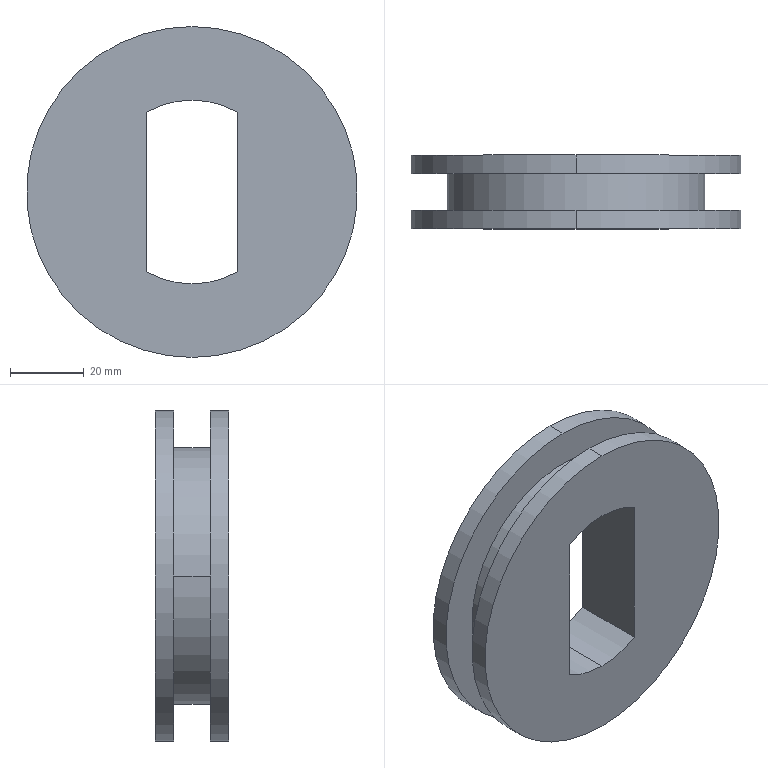Part | SolidWorks | 1 solid | 15 faces | box 90 x 20 x 90 mm | volume 78186 mm3 | cylinder 9 | plane 6 | commonest cylinder face diameters 90 x4 50 x3 70 x2
STEP:
#1=CARTESIAN_POINT('',(-35.,-5.,0.));
#2=VERTEX_POINT('',#1);
#3=CARTESIAN_POINT('',(35.,-5.,0.));
#4=VERTEX_POINT('',#3);
#5=CARTESIAN_POINT('',(0.,-5.,0.));
#6=DIRECTION('',(0.,1.,0.));
#7=DIRECTION('',(-1.,0.,0.));
#8=AXIS2_PLACEMENT_3D('',#5,#6,#7);
#9=CIRCLE('',#8,35.);
#10=EDGE_CURVE('',#2,#4,#9,.T.);
#11=ORIENTED_EDGE('',*,*,#10,.T.);
#12=CARTESIAN_POINT('',(35.,5.,0.));
#13=VERTEX_POINT('',#12);
#14=CARTESIAN_POINT('',(35.,10.,0.));
#15=DIRECTION('',(0.,1.,0.));
#16=VECTOR('',#15,1000.);
#17=LINE('',#14,#16);
#18=EDGE_CURVE('',#4,#13,#17,.T.);
#19=ORIENTED_EDGE('',*,*,#18,.T.);
#20=CARTESIAN_POINT('',(-35.,5.,0.));
#21=VERTEX_POINT('',#20);
#22=CARTESIAN_POINT('',(0.,5.,0.));
#23=DIRECTION('',(0.,1.,0.));
#24=DIRECTION('',(-1.,0.,0.));
#25=AXIS2_PLACEMENT_3D('',#22,#23,#24);
#26=CIRCLE('',#25,35.);
#27=EDGE_CURVE('',#21,#13,#26,.T.);
#28=ORIENTED_EDGE('',*,*,#27,.F.);
#29=CARTESIAN_POINT('',(-35.,10.,0.));
#30=DIRECTION('',(0.,1.,0.));
#31=VECTOR('',#30,1000.);
#32=LINE('',#29,#31);
#33=EDGE_CURVE('',#2,#21,#32,.T.);
#34=ORIENTED_EDGE('',*,*,#33,.F.);
#35=EDGE_LOOP('',(#11,#19,#28,#34));
#36=FACE_OUTER_BOUND('',#35,.T.);
#37=CARTESIAN_POINT('',(0.,10.,0.));
#38=DIRECTION('',(0.,1.,0.));
#39=DIRECTION('',(-1.,0.,0.));
#40=AXIS2_PLACEMENT_3D('',#37,#38,#39);
#41=CYLINDRICAL_SURFACE('',#40,35.);
#42=ADVANCED_FACE('',(#36),#41,.T.);
#43=CARTESIAN_POINT('',(12.5,10.,-21.651));
#44=VERTEX_POINT('',#43);
#45=CARTESIAN_POINT('',(0.,10.,-25.));
#46=VERTEX_POINT('',#45);
#47=CARTESIAN_POINT('',(0.,10.,0.));
#48=DIRECTION('',(0.,1.,0.));
#49=DIRECTION('',(0.,0.,1.));
#50=AXIS2_PLACEMENT_3D('',#47,#48,#49);
#51=CIRCLE('',#50,25.);
#52=EDGE_CURVE('',#44,#46,#51,.T.);
#53=ORIENTED_EDGE('',*,*,#52,.T.);
#54=CARTESIAN_POINT('',(0.,-10.,-25.));
#55=VERTEX_POINT('',#54);
#56=CARTESIAN_POINT('',(0.,10.,-25.));
#57=DIRECTION('',(0.,-1.,0.));
#58=VECTOR('',#57,1000.);
#59=LINE('',#56,#58);
#60=EDGE_CURVE('',#46,#55,#59,.T.);
#61=ORIENTED_EDGE('',*,*,#60,.T.);
#62=CARTESIAN_POINT('',(12.5,-10.,-21.651));
#63=VERTEX_POINT('',#62);
#64=CARTESIAN_POINT('',(0.,-10.,0.));
#65=DIRECTION('',(0.,1.,0.));
#66=DIRECTION('',(0.,0.,1.));
#67=AXIS2_PLACEMENT_3D('',#64,#65,#66);
#68=CIRCLE('',#67,25.);
#69=EDGE_CURVE('',#63,#55,#68,.T.);
#70=ORIENTED_EDGE('',*,*,#69,.F.);
#71=CARTESIAN_POINT('',(12.5,10.,-21.651));
#72=DIRECTION('',(0.,-1.,0.));
#73=VECTOR('',#72,1000.);
#74=LINE('',#71,#73);
#75=EDGE_CURVE('',#44,#63,#74,.T.);
#76=ORIENTED_EDGE('',*,*,#75,.F.);
#77=EDGE_LOOP('',(#53,#61,#70,#76));
#78=FACE_OUTER_BOUND('',#77,.T.);
#79=CARTESIAN_POINT('',(0.,10.,0.));
#80=DIRECTION('',(0.,-1.,0.));
#81=DIRECTION('',(0.,0.,-1.));
#82=AXIS2_PLACEMENT_3D('',#79,#80,#81);
#83=CYLINDRICAL_SURFACE('',#82,25.);
#84=ADVANCED_FACE('',(#78),#83,.F.);
#85=CARTESIAN_POINT('',(0.,-5.,45.));
#86=VERTEX_POINT('',#85);
#87=CARTESIAN_POINT('',(0.,-5.,-45.));
#88=VERTEX_POINT('',#87);
#89=CARTESIAN_POINT('',(0.,-5.,0.));
#90=DIRECTION('',(0.,1.,0.));
#91=DIRECTION('',(-1.,0.,0.));
#92=AXIS2_PLACEMENT_3D('',#89,#90,#91);
#93=CIRCLE('',#92,45.);
#94=EDGE_CURVE('',#86,#88,#93,.T.);
#95=ORIENTED_EDGE('',*,*,#94,.F.);
#96=CARTESIAN_POINT('',(0.,-10.,45.));
#97=VERTEX_POINT('',#96);
#98=CARTESIAN_POINT('',(0.,10.,45.));
#99=DIRECTION('',(0.,-1.,0.));
#100=VECTOR('',#99,1000.);
#101=LINE('',#98,#100);
#102=EDGE_CURVE('',#86,#97,#101,.T.);
#103=ORIENTED_EDGE('',*,*,#102,.T.);
#104=CARTESIAN_POINT('',(0.,-10.,-45.));
#105=VERTEX_POINT('',#104);
#106=CARTESIAN_POINT('',(0.,-10.,0.));
#107=DIRECTION('',(0.,1.,0.));
#108=DIRECTION('',(0.,0.,1.));
#109=AXIS2_PLACEMENT_3D('',#106,#107,#108);
#110=CIRCLE('',#109,45.);
#111=EDGE_CURVE('',#97,#105,#110,.T.);
#112=ORIENTED_EDGE('',*,*,#111,.T.);
#113=CARTESIAN_POINT('',(0.,10.,-45.));
#114=DIRECTION('',(0.,-1.,0.));
#115=VECTOR('',#114,1000.);
#116=LINE('',#113,#115);
#117=EDGE_CURVE('',#88,#105,#116,.T.);
#118=ORIENTED_EDGE('',*,*,#117,.F.);
#119=EDGE_LOOP('',(#95,#103,#112,#118));
#120=FACE_OUTER_BOUND('',#119,.T.);
#121=CARTESIAN_POINT('',(0.,10.,0.));
#122=DIRECTION('',(0.,-1.,0.));
#123=DIRECTION('',(0.,0.,-1.));
#124=AXIS2_PLACEMENT_3D('',#121,#122,#123);
#125=CYLINDRICAL_SURFACE('',#124,45.);
#126=ADVANCED_FACE('',(#120),#125,.T.);
#127=CARTESIAN_POINT('',(0.,10.,45.));
#128=VERTEX_POINT('',#127);
#129=CARTESIAN_POINT('',(0.,10.,-45.));
#130=VERTEX_POINT('',#129);
#131=CARTESIAN_POINT('',(0.,10.,0.));
#132=DIRECTION('',(0.,1.,0.));
#133=DIRECTION('',(0.,0.,1.));
#134=AXIS2_PLACEMENT_3D('',#131,#132,#133);
#135=CIRCLE('',#134,45.);
#136=EDGE_CURVE('',#128,#130,#135,.T.);
#137=ORIENTED_EDGE('',*,*,#136,.F.);
#138=CARTESIAN_POINT('',(0.,5.,45.));
#139=VERTEX_POINT('',#138);
#140=CARTESIAN_POINT('',(0.,10.,45.));
#141=DIRECTION('',(0.,-1.,0.));
#142=VECTOR('',#141,1000.);
#143=LINE('',#140,#142);
#144=EDGE_CURVE('',#128,#139,#143,.T.);
#145=ORIENTED_EDGE('',*,*,#144,.T.);
#146=CARTESIAN_POINT('',(0.,5.,-45.));
#147=VERTEX_POINT('',#146);
#148=CARTESIAN_POINT('',(0.,5.,0.));
#149=DIRECTION('',(0.,-1.,0.));
#150=DIRECTION('',(1.,0.,0.));
#151=AXIS2_PLACEMENT_3D('',#148,#149,#150);
#152=CIRCLE('',#151,45.);
#153=EDGE_CURVE('',#147,#139,#152,.T.);
#154=ORIENTED_EDGE('',*,*,#153,.F.);
#155=CARTESIAN_POINT('',(0.,10.,-45.));
#156=DIRECTION('',(0.,-1.,0.));
#157=VECTOR('',#156,1000.);
#158=LINE('',#155,#157);
#159=EDGE_CURVE('',#130,#147,#158,.T.);
#160=ORIENTED_EDGE('',*,*,#159,.F.);
#161=EDGE_LOOP('',(#137,#145,#154,#160));
#162=FACE_OUTER_BOUND('',#161,.T.);
#163=CARTESIAN_POINT('',(0.,10.,0.));
#164=DIRECTION('',(0.,-1.,0.));
#165=DIRECTION('',(0.,0.,-1.));
#166=AXIS2_PLACEMENT_3D('',#163,#164,#165);
#167=CYLINDRICAL_SURFACE('',#166,45.);
#168=ADVANCED_FACE('',(#162),#167,.T.);
#169=ORIENTED_EDGE('',*,*,#144,.F.);
#170=CARTESIAN_POINT('',(0.,10.,0.));
#171=DIRECTION('',(0.,1.,0.));
#172=DIRECTION('',(0.,0.,1.));
#173=AXIS2_PLACEMENT_3D('',#170,#171,#172);
#174=CIRCLE('',#173,45.);
#175=EDGE_CURVE('',#130,#128,#174,.T.);
#176=ORIENTED_EDGE('',*,*,#175,.F.);
#177=ORIENTED_EDGE('',*,*,#159,.T.);
#178=CARTESIAN_POINT('',(0.,5.,0.));
#179=DIRECTION('',(0.,-1.,0.));
#180=DIRECTION('',(1.,0.,0.));
#181=AXIS2_PLACEMENT_3D('',#178,#179,#180);
#182=CIRCLE('',#181,45.);
#183=EDGE_CURVE('',#139,#147,#182,.T.);
#184=ORIENTED_EDGE('',*,*,#183,.F.);
#185=EDGE_LOOP('',(#169,#176,#177,#184));
#186=FACE_OUTER_BOUND('',#185,.T.);
#187=CARTESIAN_POINT('',(0.,10.,0.));
#188=DIRECTION('',(0.,-1.,0.));
#189=DIRECTION('',(0.,0.,-1.));
#190=AXIS2_PLACEMENT_3D('',#187,#188,#189);
#191=CYLINDRICAL_SURFACE('',#190,45.);
#192=ADVANCED_FACE('',(#186),#191,.T.);
#193=ORIENTED_EDGE('',*,*,#102,.F.);
#194=CARTESIAN_POINT('',(0.,-5.,0.));
#195=DIRECTION('',(0.,1.,0.));
#196=DIRECTION('',(-1.,0.,0.));
#197=AXIS2_PLACEMENT_3D('',#194,#195,#196);
#198=CIRCLE('',#197,45.);
#199=EDGE_CURVE('',#88,#86,#198,.T.);
#200=ORIENTED_EDGE('',*,*,#199,.F.);
#201=ORIENTED_EDGE('',*,*,#117,.T.);
#202=CARTESIAN_POINT('',(0.,-10.,0.));
#203=DIRECTION('',(0.,1.,0.));
#204=DIRECTION('',(0.,0.,1.));
#205=AXIS2_PLACEMENT_3D('',#202,#203,#204);
#206=CIRCLE('',#205,45.);
#207=EDGE_CURVE('',#105,#97,#206,.T.);
#208=ORIENTED_EDGE('',*,*,#207,.T.);
#209=EDGE_LOOP('',(#193,#200,#201,#208));
#210=FACE_OUTER_BOUND('',#209,.T.);
#211=CARTESIAN_POINT('',(0.,10.,0.));
#212=DIRECTION('',(0.,-1.,0.));
#213=DIRECTION('',(0.,0.,-1.));
#214=AXIS2_PLACEMENT_3D('',#211,#212,#213);
#215=CYLINDRICAL_SURFACE('',#214,45.);
#216=ADVANCED_FACE('',(#210),#215,.T.);
#217=CARTESIAN_POINT('',(12.5,-10.,21.651));
#218=VERTEX_POINT('',#217);
#219=CARTESIAN_POINT('',(12.5,-10.,0.));
#220=DIRECTION('',(0.,0.,1.));
#221=VECTOR('',#220,1000.);
#222=LINE('',#219,#221);
#223=EDGE_CURVE('',#63,#218,#222,.T.);
#224=ORIENTED_EDGE('',*,*,#223,.T.);
#225=CARTESIAN_POINT('',(12.5,10.,21.651));
#226=VERTEX_POINT('',#225);
#227=CARTESIAN_POINT('',(12.5,10.,21.651));
#228=DIRECTION('',(0.,-1.,0.));
#229=VECTOR('',#228,1000.);
#230=LINE('',#227,#229);
#231=EDGE_CURVE('',#226,#218,#230,.T.);
#232=ORIENTED_EDGE('',*,*,#231,.F.);
#233=CARTESIAN_POINT('',(12.5,10.,0.));
#234=DIRECTION('',(0.,0.,1.));
#235=VECTOR('',#234,1000.);
#236=LINE('',#233,#235);
#237=EDGE_CURVE('',#44,#226,#236,.T.);
#238=ORIENTED_EDGE('',*,*,#237,.F.);
#239=ORIENTED_EDGE('',*,*,#75,.T.);
#240=EDGE_LOOP('',(#224,#232,#238,#239));
#241=FACE_OUTER_BOUND('',#240,.T.);
#242=CARTESIAN_POINT('',(12.5,10.,0.));
#243=DIRECTION('',(1.,0.,0.));
#244=DIRECTION('',(0.,0.,-1.));
#245=AXIS2_PLACEMENT_3D('',#242,#243,#244);
#246=PLANE('',#245);
#247=ADVANCED_FACE('',(#241),#246,.F.);
#248=CARTESIAN_POINT('',(-12.5,-10.,21.651));
#249=VERTEX_POINT('',#248);
#250=CARTESIAN_POINT('',(0.,-10.,0.));
#251=DIRECTION('',(0.,1.,0.));
#252=DIRECTION('',(0.,0.,1.));
#253=AXIS2_PLACEMENT_3D('',#250,#251,#252);
#254=CIRCLE('',#253,25.);
#255=EDGE_CURVE('',#249,#218,#254,.T.);
#256=ORIENTED_EDGE('',*,*,#255,.F.);
#257=CARTESIAN_POINT('',(-12.5,10.,21.651));
#258=VERTEX_POINT('',#257);
#259=CARTESIAN_POINT('',(-12.5,10.,21.651));
#260=DIRECTION('',(0.,-1.,0.));
#261=VECTOR('',#260,1000.);
#262=LINE('',#259,#261);
#263=EDGE_CURVE('',#258,#249,#262,.T.);
#264=ORIENTED_EDGE('',*,*,#263,.F.);
#265=CARTESIAN_POINT('',(0.,10.,0.));
#266=DIRECTION('',(0.,1.,0.));
#267=DIRECTION('',(0.,0.,1.));
#268=AXIS2_PLACEMENT_3D('',#265,#266,#267);
#269=CIRCLE('',#268,25.);
#270=EDGE_CURVE('',#258,#226,#269,.T.);
#271=ORIENTED_EDGE('',*,*,#270,.T.);
#272=ORIENTED_EDGE('',*,*,#231,.T.);
#273=EDGE_LOOP('',(#256,#264,#271,#272));
#274=FACE_OUTER_BOUND('',#273,.T.);
#275=CARTESIAN_POINT('',(0.,10.,0.));
#276=DIRECTION('',(0.,-1.,0.));
#277=DIRECTION('',(0.,0.,-1.));
#278=AXIS2_PLACEMENT_3D('',#275,#276,#277);
#279=CYLINDRICAL_SURFACE('',#278,25.);
#280=ADVANCED_FACE('',(#274),#279,.F.);
#281=CARTESIAN_POINT('',(-12.5,-10.,-21.651));
#282=VERTEX_POINT('',#281);
#283=CARTESIAN_POINT('',(-12.5,-10.,0.));
#284=DIRECTION('',(0.,0.,1.));
#285=VECTOR('',#284,1000.);
#286=LINE('',#283,#285);
#287=EDGE_CURVE('',#282,#249,#286,.T.);
#288=ORIENTED_EDGE('',*,*,#287,.F.);
#289=CARTESIAN_POINT('',(-12.5,10.,-21.651));
#290=VERTEX_POINT('',#289);
#291=CARTESIAN_POINT('',(-12.5,10.,-21.651));
#292=DIRECTION('',(0.,-1.,0.));
#293=VECTOR('',#292,1000.);
#294=LINE('',#291,#293);
#295=EDGE_CURVE('',#290,#282,#294,.T.);
#296=ORIENTED_EDGE('',*,*,#295,.F.);
#297=CARTESIAN_POINT('',(-12.5,10.,0.));
#298=DIRECTION('',(0.,0.,1.));
#299=VECTOR('',#298,1000.);
#300=LINE('',#297,#299);
#301=EDGE_CURVE('',#290,#258,#300,.T.);
#302=ORIENTED_EDGE('',*,*,#301,.T.);
#303=ORIENTED_EDGE('',*,*,#263,.T.);
#304=EDGE_LOOP('',(#288,#296,#302,#303));
#305=FACE_OUTER_BOUND('',#304,.T.);
#306=CARTESIAN_POINT('',(-12.5,10.,0.));
#307=DIRECTION('',(1.,0.,0.));
#308=DIRECTION('',(0.,0.,-1.));
#309=AXIS2_PLACEMENT_3D('',#306,#307,#308);
#310=PLANE('',#309);
#311=ADVANCED_FACE('',(#305),#310,.T.);
#312=ORIENTED_EDGE('',*,*,#60,.F.);
#313=CARTESIAN_POINT('',(0.,10.,0.));
#314=DIRECTION('',(0.,1.,0.));
#315=DIRECTION('',(0.,0.,1.));
#316=AXIS2_PLACEMENT_3D('',#313,#314,#315);
#317=CIRCLE('',#316,25.);
#318=EDGE_CURVE('',#46,#290,#317,.T.);
#319=ORIENTED_EDGE('',*,*,#318,.T.);
#320=ORIENTED_EDGE('',*,*,#295,.T.);
#321=CARTESIAN_POINT('',(0.,-10.,0.));
#322=DIRECTION('',(0.,1.,0.));
#323=DIRECTION('',(0.,0.,1.));
#324=AXIS2_PLACEMENT_3D('',#321,#322,#323);
#325=CIRCLE('',#324,25.);
#326=EDGE_CURVE('',#55,#282,#325,.T.);
#327=ORIENTED_EDGE('',*,*,#326,.F.);
#328=EDGE_LOOP('',(#312,#319,#320,#327));
#329=FACE_OUTER_BOUND('',#328,.T.);
#330=CARTESIAN_POINT('',(0.,10.,0.));
#331=DIRECTION('',(0.,-1.,0.));
#332=DIRECTION('',(0.,0.,-1.));
#333=AXIS2_PLACEMENT_3D('',#330,#331,#332);
#334=CYLINDRICAL_SURFACE('',#333,25.);
#335=ADVANCED_FACE('',(#329),#334,.F.);
#336=ORIENTED_EDGE('',*,*,#237,.T.);
#337=ORIENTED_EDGE('',*,*,#270,.F.);
#338=ORIENTED_EDGE('',*,*,#301,.F.);
#339=ORIENTED_EDGE('',*,*,#318,.F.);
#340=ORIENTED_EDGE('',*,*,#52,.F.);
#341=EDGE_LOOP('',(#336,#337,#338,#339,#340));
#342=FACE_BOUND('',#341,.T.);
#343=ORIENTED_EDGE('',*,*,#175,.T.);
#344=ORIENTED_EDGE('',*,*,#136,.T.);
#345=EDGE_LOOP('',(#343,#344));
#346=FACE_OUTER_BOUND('',#345,.T.);
#347=CARTESIAN_POINT('',(0.,10.,0.));
#348=DIRECTION('',(0.,1.,0.));
#349=DIRECTION('',(0.,0.,1.));
#350=AXIS2_PLACEMENT_3D('',#347,#348,#349);
#351=PLANE('',#350);
#352=ADVANCED_FACE('',(#342,#346),#351,.T.);
#353=ORIENTED_EDGE('',*,*,#223,.F.);
#354=ORIENTED_EDGE('',*,*,#69,.T.);
#355=ORIENTED_EDGE('',*,*,#326,.T.);
#356=ORIENTED_EDGE('',*,*,#287,.T.);
#357=ORIENTED_EDGE('',*,*,#255,.T.);
#358=EDGE_LOOP('',(#353,#354,#355,#356,#357));
#359=FACE_BOUND('',#358,.T.);
#360=ORIENTED_EDGE('',*,*,#207,.F.);
#361=ORIENTED_EDGE('',*,*,#111,.F.);
#362=EDGE_LOOP('',(#360,#361));
#363=FACE_OUTER_BOUND('',#362,.T.);
#364=CARTESIAN_POINT('',(0.,-10.,0.));
#365=DIRECTION('',(0.,1.,0.));
#366=DIRECTION('',(0.,0.,1.));
#367=AXIS2_PLACEMENT_3D('',#364,#365,#366);
#368=PLANE('',#367);
#369=ADVANCED_FACE('',(#359,#363),#368,.F.);
#370=ORIENTED_EDGE('',*,*,#27,.T.);
#371=CARTESIAN_POINT('',(0.,5.,0.));
#372=DIRECTION('',(0.,1.,0.));
#373=DIRECTION('',(-1.,0.,0.));
#374=AXIS2_PLACEMENT_3D('',#371,#372,#373);
#375=CIRCLE('',#374,35.);
#376=EDGE_CURVE('',#13,#21,#375,.T.);
#377=ORIENTED_EDGE('',*,*,#376,.T.);
#378=EDGE_LOOP('',(#370,#377));
#379=FACE_BOUND('',#378,.T.);
#380=ORIENTED_EDGE('',*,*,#153,.T.);
#381=ORIENTED_EDGE('',*,*,#183,.T.);
#382=EDGE_LOOP('',(#380,#381));
#383=FACE_OUTER_BOUND('',#382,.T.);
#384=CARTESIAN_POINT('',(35.,5.,0.));
#385=DIRECTION('',(0.,-1.,0.));
#386=DIRECTION('',(1.,0.,0.));
#387=AXIS2_PLACEMENT_3D('',#384,#385,#386);
#388=PLANE('',#387);
#389=ADVANCED_FACE('',(#379,#383),#388,.T.);
#390=ORIENTED_EDGE('',*,*,#10,.F.);
#391=CARTESIAN_POINT('',(0.,-5.,0.));
#392=DIRECTION('',(0.,1.,0.));
#393=DIRECTION('',(-1.,0.,0.));
#394=AXIS2_PLACEMENT_3D('',#391,#392,#393);
#395=CIRCLE('',#394,35.);
#396=EDGE_CURVE('',#4,#2,#395,.T.);
#397=ORIENTED_EDGE('',*,*,#396,.F.);
#398=EDGE_LOOP('',(#390,#397));
#399=FACE_BOUND('',#398,.T.);
#400=ORIENTED_EDGE('',*,*,#199,.T.);
#401=ORIENTED_EDGE('',*,*,#94,.T.);
#402=EDGE_LOOP('',(#400,#401));
#403=FACE_OUTER_BOUND('',#402,.T.);
#404=CARTESIAN_POINT('',(35.,-5.,0.));
#405=DIRECTION('',(0.,1.,0.));
#406=DIRECTION('',(-1.,0.,0.));
#407=AXIS2_PLACEMENT_3D('',#404,#405,#406);
#408=PLANE('',#407);
#409=ADVANCED_FACE('',(#399,#403),#408,.T.);
#410=ORIENTED_EDGE('',*,*,#18,.F.);
#411=ORIENTED_EDGE('',*,*,#396,.T.);
#412=ORIENTED_EDGE('',*,*,#33,.T.);
#413=ORIENTED_EDGE('',*,*,#376,.F.);
#414=EDGE_LOOP('',(#410,#411,#412,#413));
#415=FACE_OUTER_BOUND('',#414,.T.);
#416=CARTESIAN_POINT('',(0.,10.,0.));
#417=DIRECTION('',(0.,1.,0.));
#418=DIRECTION('',(-1.,0.,0.));
#419=AXIS2_PLACEMENT_3D('',#416,#417,#418);
#420=CYLINDRICAL_SURFACE('',#419,35.);
#421=ADVANCED_FACE('',(#415),#420,.T.);
#422=CLOSED_SHELL('',(#42,#84,#126,#168,#192,#216,#247,#280,#311,#335,#352,#369,#389,#409,#421));
#423=MANIFOLD_SOLID_BREP('',#422);
#424=CARTESIAN_POINT('',(0.,0.,0.));
#425=DIRECTION('',(0.,0.,1.));
#426=DIRECTION('',(1.,0.,0.));
#427=AXIS2_PLACEMENT_3D('',#424,#425,#426);
#428=(LENGTH_UNIT()NAMED_UNIT(*)SI_UNIT(.MILLI.,.METRE.));
#429=UNCERTAINTY_MEASURE_WITH_UNIT(LENGTH_MEASURE(0.00001),#428,'','');
#430=(NAMED_UNIT(*)PLANE_ANGLE_UNIT()SI_UNIT($,.RADIAN.));
#431=(NAMED_UNIT(*)SI_UNIT($,.STERADIAN.)SOLID_ANGLE_UNIT());
#432=(GEOMETRIC_REPRESENTATION_CONTEXT(3)GLOBAL_UNCERTAINTY_ASSIGNED_CONTEXT((#429))GLOBAL_UNIT_ASSIGNED_CONTEXT((#428,#430,#431))REPRESENTATION_CONTEXT('',''));
#433=ADVANCED_BREP_SHAPE_REPRESENTATION('',(#423,#427),#432);